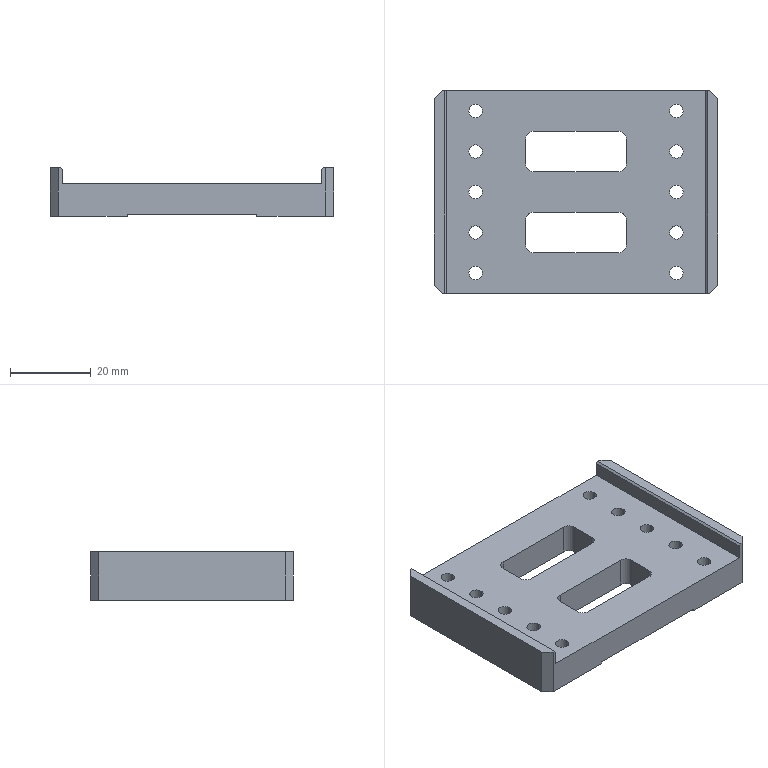Part | SolidWorks | features Chamfer 2, ICE 2, Cut 1, Extrusion 1, Fillet 1, HoleWzd 1, LPattern 1, MirrorPattern 1 | 1 solid | 56 faces | box 70 x 50 x 12 mm | volume 23909 mm3 | cylinder 28 | plane 28 | commonest cylinder face diameters 3.3 x20 4 x8